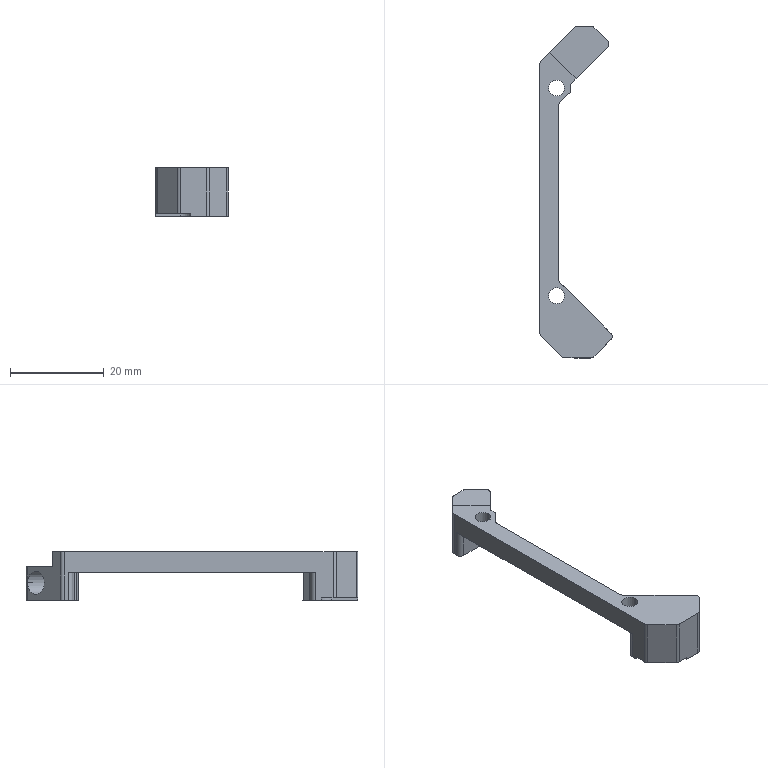NC program | NX | posted with a generic post | part box 15.463 x 71 x 10.4 mm
Whole program:
N10 G17 G21 G94 G90
(PLANAR_MILL_1_COPY_1 , TOOL : D2-ROUGHING)
N12 T03 M6
N14 G54
N16 G17 G0 G90 X-16.548 Y2.282 S4000 M3
N18 G43 Z50. H3
N20 Z2.
N22 G94 G1 Z-1. F800.
N24 G3 X-16.948 Y2.682 R0.4
N26 G1 X-18.588
N28 X-19.747 Y1.522
N30 G3 X-19.747 Y0.957 R0.4
N32 G1 Z2.
N34 G0 Z3.
N36 X-16.548 Y2.282
N38 Z1.
N40 G1 Z-2.
N42 G3 X-16.948 Y2.682 R0.4
N44 G1 X-18.588
N46 X-19.747 Y1.522
N48 G3 X-19.747 Y0.957 R0.4
N50 G1 Z1.
N52 G0 Z2.
N54 X-16.548 Y2.282
N56 Z0.
N58 G1 Z-3.
N60 G3 X-16.948 Y2.682 R0.4
N62 G1 X-18.588
N64 X-19.747 Y1.522
N66 G3 X-19.747 Y0.957 R0.4
N68 G1 Z0.
N70 G0 Z1.
N72 X-16.548 Y2.282
N74 Z-1.
N76 G1 Z-4.
N78 G3 X-16.948 Y2.682 R0.4
N80 G1 X-18.588
N82 X-19.747 Y1.522
N84 G3 X-19.747 Y0.957 R0.4
N86 G1 Z-1.
N88 G0 Z0.
N90 X-16.548 Y2.282
N92 Z-1.9
N94 G1 Z-4.9
N96 G3 X-16.948 Y2.682 R0.4
N98 G1 X-18.588
N100 X-19.747 Y1.522
N102 G3 X-19.747 Y0.957 R0.4
N104 G1 Z-1.9
N106 G0 Z50.
(PLANAR_MILL_1_COPY , TOOL : D2-ROUGHING)
N108 X23.325 Y-1.325
N110 Z-1.9
N112 G1 Z-4.9 F150.
N114 G41 X23.407 Y-1.268 D3
N116 G3 X23.407 Y-0.702 R0.4
N118 G1 X22.533 Y0.172
N120 X21.548
N122 G3 X21.148 Y-0.228 R0.4
N124 G40
N126 G1 X21.165 Y-0.327
N128 Z-1.9
N130 G0 Z3.
N132 X23.336 Y-1.314
N134 Z-1.9
N136 G1 Z-4.9
N138 G41 X23.418 Y-1.257
N140 G3 X23.418 Y-0.691 R0.4
N142 G1 X22.54 Y0.187
N144 X21.548
N146 G3 X21.148 Y-0.213 R0.4
N148 G40
N150 G1 X21.165 Y-0.312
N152 Z-1.9
N154 G0 Z3.
N156 X19.212 Y1.094
N158 Z-1.9
N160 G1 Z-4.9
N162 G41 X19.294 Y1.151
N164 G3 X19.294 Y1.717 R0.4
N166 G1 X18.314 Y2.697
N168 X16.928
N170 G3 X16.528 Y2.297 R0.4
N172 G40
N174 G1 X16.546 Y2.198
N176 Z-1.9
N178 G0 Z3.
N180 X19.222 Y1.105
N182 Z-1.9
N184 G1 Z-4.9
N186 G41 X19.304 Y1.162
N188 G3 X19.304 Y1.728 R0.4
N190 G1 X18.32 Y2.712
N192 X16.928
N194 G3 X16.528 Y2.312 R0.4
N196 G40
N198 G1 X16.546 Y2.213
N200 Z-1.9
N202 G0 Z3.
N204 X-16.826 Y2.198
N206 Z-1.9
N208 G1 Z-4.9
N210 G41 X-16.809 Y2.297
N212 G3 X-17.209 Y2.697 R0.4
N214 G1 X-18.594
N216 X-19.574 Y1.717
N218 G3 X-19.574 Y1.151 R0.4
N220 G40
N222 G1 X-19.492 Y1.094
N224 Z-1.9
N226 G0 Z3.
N228 X-16.826 Y2.213
N230 Z-1.9
N232 G1 Z-4.9
N234 G41 X-16.809 Y2.312
N236 G3 X-17.209 Y2.712 R0.4
N238 G1 X-18.6
N240 X-19.585 Y1.728
N242 G3 X-19.585 Y1.162 R0.4
N244 G40
N246 G1 X-19.503 Y1.105
N248 Z-1.9
N250 G0 Z50.
N252 M5
(FLOOR_FACING_1 , TOOL : D54-面刀)
N254 T01 M6
N256 G54
N258 G17 G0 G90 X63.5 Y-0.232 S4500 M3
N260 G43 Z55. H1
N262 Z7.02
N264 G94 G1 Z4.02 F2000.
N266 X60.5
N268 X-60.5
N270 X-63.5
N272 Z7.02
N274 G0 Z55.
N276 X63.5
N278 Z6.04
N280 G1 Z3.04
N282 X60.5
N284 X-60.5
N286 X-63.5
N288 Z6.04
N290 G0 Z55.
N292 X63.5
N294 Z5.06
N296 G1 Z2.06
N298 X60.5
N300 X-60.5
N302 X-63.5
N304 Z5.06
N306 G0 Z55.
N308 X63.5
N310 Z4.08
N312 G1 Z1.08
N314 X60.5
N316 X-60.5
N318 X-63.5
N320 Z4.08
N322 G0 Z55.
N324 X63.5
N326 Z3.1
N328 G1 Z0.1
N330 X60.5
N332 X-60.5
N334 X-63.5
N336 Z3.1
N338 G0 Z55.
(CAVITY_MILL , TOOL : D8-ROUGHING)
N340 T02 M6
N342 G17 G43 G0 G90 X-4.013 Y11.792 Z50.1 S5000 H2 M3
N344 Z1.525
N346 G94 G1 Z-1.475 F2500.
N348 G3 X-0.013 Y7.792 R4.
N350 G1 X20.899
N352 X21.421 Y7.793
N354 G2 X25.216 Y11.732 R5.199
N356 G1 X25.494
N358 G3 X21.4 Y6.732 R5.1
N360 G1 Y3.486
N362 X21.042 Y3.127
N364 G3 X21.004 Y-4.048 R5.1
N366 G1 X20.961 Y-4.095
N368 X20.919 Y-4.046
N370 G2 X19.978 Y1.723 R5.159
N372 G1 X19.979 Y1.761
N374 X19.988 Y1.79
N376 X20.153 Y2.058
N378 X20.328 Y2.342
N380 X19.938 Y2.731
N382 X19.239 Y3.429
N384 X19.137 Y3.509
N386 X18.914 Y3.634
N388 X18.653 Y3.671
N390 X-17.966 Y3.672
N392 X-18.402 Y3.669
N394 X-18.521 Y3.652
N396 X-18.821 Y3.568
N398 X-20.451 Y1.922
N400 X-20.401 Y1.775
N402 G2 X-21.718 Y-3.43 R5.153
N404 G1 X-21.76 Y-3.467
N406 X-21.791 Y-3.421
N408 X-21.749 Y-3.378
N410 G3 X-21.4 Y3.448 R5.1
N412 G1 Y6.732
N414 G3 X-25.487 Y11.73 R5.1
N416 G1 X-25.224
N418 G2 X-21.448 Y7.792 R5.174
N420 G1 X-0.013
N422 G3 X3.987 Y11.792 R4.
N424 G1 Z1.525
N426 G0 Z50.1
N428 X-4.013
N430 Z0.05
N432 G1 Z-2.95
N434 G3 X-0.013 Y7.792 R4.
N436 G1 X20.899
N438 X21.421 Y7.793
N440 G2 X25.216 Y11.732 R5.199
N442 G1 X25.495
N444 G3 X21.4 Y6.732 R5.1
N446 G1 Y3.486
N448 X21.042 Y3.127
N450 G3 X21.004 Y-4.048 R5.1
N452 G1 X20.961 Y-4.095
N454 X20.919 Y-4.046
N456 G2 X19.978 Y1.723 R5.159
N458 G1 X19.979 Y1.761
N460 X19.988 Y1.79
N462 X20.328 Y2.342
N464 X19.239 Y3.429
N466 X19.137 Y3.509
N468 X18.914 Y3.634
N470 X18.653 Y3.671
N472 X-17.966 Y3.672
N474 X-18.402 Y3.669
N476 X-18.521 Y3.652
N478 X-18.821 Y3.568
N480 X-20.451 Y1.922
N482 X-20.401 Y1.775
N484 G2 X-21.707 Y-3.421 R5.153
N486 G1 X-21.749 Y-3.468
N488 X-21.791 Y-3.421
N490 X-21.749 Y-3.378
N492 G3 X-21.4 Y3.448 R5.1
N494 G1 Y6.732
N496 G3 X-25.487 Y11.73 R5.1
N498 G1 X-25.224
N500 G2 X-21.448 Y7.792 R5.174
N502 G1 X-0.013
N504 G3 X3.987 Y11.792 R4.
N506 G1 Z0.05
N508 G0 Z50.1
N510 X-4.013
N512 Z-1.425
N514 G1 Z-4.425
N516 G3 X-0.013 Y7.792 R4.
N518 G1 X20.899
N520 X21.421 Y7.793
N522 G2 X25.216 Y11.732 R5.199
N524 G1 X25.495
N526 G3 X21.4 Y6.732 R5.1
N528 G1 Y3.486
N530 X21.042 Y3.127
N532 G3 X21.004 Y-4.048 R5.1
N534 G1 X20.961 Y-4.095
N536 X20.919 Y-4.046
N538 G2 X19.978 Y1.723 R5.159
N540 G1 X19.979 Y1.761
N542 X19.988 Y1.79
N544 X20.153 Y2.058
N546 X20.328 Y2.342
N548 X19.239 Y3.429
N550 X19.137 Y3.509
N552 X18.914 Y3.634
N554 X18.653 Y3.671
N556 X-17.966 Y3.672
N558 X-18.402 Y3.669
N560 X-18.521 Y3.652
N562 X-18.821 Y3.568
N564 X-20.451 Y1.922
N566 X-20.401 Y1.775
N568 G2 X-21.707 Y-3.421 R5.153
N570 G1 X-21.749 Y-3.468
N572 X-21.791 Y-3.421
N574 X-21.749 Y-3.378
N576 G3 X-21.4 Y3.448 R5.1
N578 G1 Y6.732
N580 G3 X-25.488 Y11.73 R5.1
N582 G1 X-25.225
N584 G2 X-21.448 Y7.792 R5.174
N586 G1 X-0.013
N588 G3 X3.987 Y11.792 R4.
N590 G1 Z-1.425
N592 G0 Z50.1
N594 X-4.013
N596 Z-2.9
N598 G1 Z-5.9
N600 G3 X-0.013 Y7.792 R4.
N602 G1 X20.899
N604 X21.421 Y7.793
N606 G2 X21.719 Y8.732 R5.199
N608 X25.217 Y11.732 R5.199
N610 G1 X25.495
N612 G3 X21.4 Y6.732 R5.1
N614 G1 Y3.486
N616 X21.042 Y3.127
N618 G3 X21.004 Y-4.048 R5.1
N620 G1 X20.961 Y-4.095
N622 X20.919 Y-4.046
N624 G2 X19.978 Y1.723 R5.159
N626 G1 X19.979 Y1.761
N628 X19.988 Y1.79
N630 X20.328 Y2.342
N632 X19.938 Y2.731
N634 X19.239 Y3.429
N636 X19.137 Y3.509
N638 X18.914 Y3.634
N640 X18.653 Y3.671
N642 X-17.966 Y3.672
N644 X-18.402 Y3.669
N646 X-18.521 Y3.652
N648 X-18.821 Y3.568
N650 X-20.054 Y2.323
N652 X-20.451 Y1.922
N654 X-20.401 Y1.775
N656 G2 X-21.707 Y-3.421 R5.153
N658 G1 X-21.749 Y-3.468
N660 X-21.791 Y-3.421
N662 X-21.749 Y-3.378
N664 G3 X-21.4 Y3.448 R5.1
N666 G1 Y6.732
N668 G3 X-25.488 Y11.73 R5.1
N670 G1 X-25.225
N672 G2 X-21.448 Y7.792 R5.174
N674 G1 X-0.013
N676 G3 X3.987 Y11.792 R4.
N678 G1 Z-2.9
N680 G0 Z50.1
N682 M5
(PLANAR_MILL_4 , TOOL : D8-FINISHING)
N684 T04 M6
N686 G54
N688 G17 G0 G90 X-26.5 Y16.732 S4500 M3
N690 G43 Z50. H4
N692 Z-3.
N694 G94 G1 Z-6. F700.
N696 Y11.732
N698 G2 X-21.5 Y6.732 R5.
N700 G1 Y3.412
N702 G2 X-21.819 Y-3.307 R5.
N704 G1 X-18.284 Y-6.843
N706 Z-3.
N708 G0 Z50.
N710 X17.577 Y-7.55
N712 Z-3.
N714 G1 Z-6.
N716 X21.112 Y-4.015
N718 G2 X21.112 Y3.057 R5.
N720 G1 X21.5 Y3.444
N722 Y6.732
N724 G2 X26.5 Y11.732 R5.
N726 G1 Y16.732
N728 Z-3.
N730 G0 Z50.
(PLANAR_MILL_4_COPY_COPY , TOOL : D4-FINISHING)
N732 T07 M6
N734 G17 G43 G0 G90 X34.97 Y7.583 Z50.1 S4500 H7 M3
N736 Z2.6
N738 G94 G1 Z-0.4 F1000.
N740 X32.849 Y5.462
N742 X35.207 Y3.104
N744 G2 X35.5 Y2.352 R1.001
N746 G1 X29.839
N748 X29.774 Y2.339
N750 X29.726 Y2.387
N752 X29.739 Y2.452
N754 Y7.732
N756 X30.165
N758 G2 X30.872 Y7.439 R1.
N760 G1 X32.849 Y5.462
N762 X31.718 Y4.331
N764 X32.096 Y3.952
N766 X31.339
N768 Y4.709
N770 X31.718 Y4.331
N772 Z1.6
N774 G0 Z50.1
(PLANAR_MILL_4_COPY_COPY_COPY , TOOL : D4-FINISHING)
N776 X34.97 Y7.583
N778 Z50.
N780 Z2.5
N782 G1 Z-0.5 F500.
N784 X32.849 Y5.462
N786 X35.207 Y3.104
N788 G2 X35.5 Y2.397 R1.
N790 G1 Y2.252
N792 X29.839
N794 G2 X29.639 Y2.452 R0.2
N796 G1 Y7.732
N798 X30.165
N800 G2 X30.872 Y7.439 R1.
N802 G1 X32.849 Y5.462
N804 X31.718 Y4.331
N806 X32.196 Y3.852
N808 X31.239
N810 Y4.809
N812 X31.718 Y4.331
N814 Z1.5
N816 G0 Z50.
N818 M5
(PLANAR_MILL_5_COPY , TOOL : D4倒角刀)
N820 T05 M6
N822 G54
N824 G17 G0 G90 X-36.621 Y-6.668 S4500 M3
N826 G43 Z50. H5
N828 Z2.
N830 G94 G1 Z-1. F1000.
N832 X-35.914 Y-5.961
N834 G3 X-35.914 Y-4.546 R1.
N836 G2 X-36.5 Y-3.132 R2.
N838 G1 Y-0.432
N840 G2 X-35.914 Y0.983 R2.
N842 G1 X-28.751 Y8.146
N844 G2 X-27.337 Y8.732 R2.
N846 G1 X-26.5
N848 G2 X-24.5 Y6.732 R2.
N850 G1 Y2.201
N852 X-23.941 Y1.642
N854 G2 X-23.941 Y-1.186 R2.
N856 G1 X-30.193 Y-7.439
N858 G2 X-33.022 Y-7.439 R2.
N860 G1 X-35.914 Y-4.546
N862 G3 X-37.328 Y-4.546 R1.
N864 G1 X-37.946 Y-5.164
N866 Z2.
N868 G0 Z50.
(PLANAR_MILL_5_COPY_COPY , TOOL : D4倒角刀)
N870 X20.023 Y-1.511
N872 Z-4.
N874 G1 Z-7.
N876 X21.437 Y-0.097
N878 X18.609 Y2.732
N880 X-18.328
N882 X-20.268 Y0.792
N884 G2 X-21.682 Y0.207 R2.
N886 G1 Y-1.793
N888 Z-4.
N890 G0 Z50.
N892 X-23.5 Y10.732
N894 Z-4.
N896 G1 Z-7.
N898 Y8.732
N900 X23.5
N902 Y10.732
N904 Z-4.
N906 G0 Z50.
(FLOOR_WALL_COPY_COPY_COPY , TOOL : D2-ROUGHING)
N908 T03 M6
N910 G17 G43 G0 G90 X-18.504 Y5.26 Z20. S5000 H3 M3
N912 Z-0.395
N914 G94 G1 Z-3.395 F800.
N916 G41 X-18.521 Y5.162 D3
N918 G3 X-18.121 Y4.762 R0.4
N920 G1 X18.402
N922 G2 X20.191 Y4.021 R2.53
N924 G1 X30.901 Y-6.687
N926 X34.47 Y-3.082
N928 X34.466 Y2.383
N930 X34.443 Y2.411
N932 X30.114 Y6.702
N934 X-27.351 Y6.675
N936 X-34.47 Y-0.482
N938 Y-3.082
N940 X-34.462 Y-3.123
N942 X-31.608 Y-5.98
N944 X-23.983 Y1.642
N946 G2 X-22.548 Y2.237 R2.03
N948 G1 X-21.667 Y2.264
N950 X-19.91 Y4.021
N952 G2 X-18.121 Y4.762 R2.53
N954 G1 X-17.121
N956 G3 X-16.721 Y5.162 R0.4
N958 G40
N960 G1 X-16.739 Y5.26
N962 Z-0.395
N964 G0 Z20.
N966 M5
(PLANAR_MILL_6_COPY , TOOL : D4-FINISHING)
N968 T07 M6
N970 G54
N972 G17 G0 G90 X5.765 Y-0.637 S4000 M3
N974 G43 Z50. H7
N976 Z-2.55
N978 G94 G1 Z-5.55 F200.
N980 G41 X5.8 Y-0.44 D7
N982 G3 X5.5 Y-0.14 R0.3
N984 X4.19 Y-1.45 R1.31
N986 X5.5 Y-0.14 R-1.31
N988 X5.2 Y-0.44 R0.3
N990 G40
N992 G1 X5.235 Y-0.637
N994 X5.765 Y-0.627
N996 G41 X5.8 Y-0.43
N998 G3 X5.5 Y-0.13 R0.3
N1000 X4.18 Y-1.45 R1.32
N1002 X5.5 Y-0.13 R-1.32
N1004 X5.2 Y-0.43 R0.3
N1006 G40
N1008 G1 X5.235 Y-0.627
N1010 Z-3.55
N1012 G0 Z50.
N1014 M5
N1016 M2